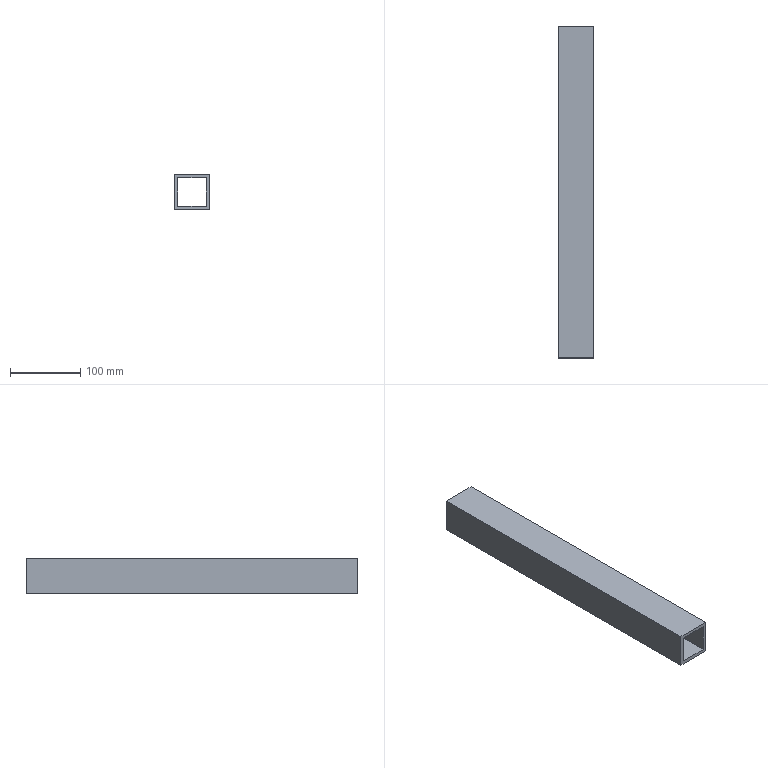Part | NX | features solid 2 | 1 solid | 10 faces | box 50 x 473 x 50 mm | volume 425700 mm3 | plane 10
STEP:
#1=CARTESIAN_POINT('',(1105.,523.,-520.));
#2=VERTEX_POINT('',#1);
#3=CARTESIAN_POINT('',(1105.,523.,-560.));
#4=VERTEX_POINT('',#3);
#5=CARTESIAN_POINT('',(1105.,523.,-520.));
#6=DIRECTION('',(0.,0.,-1.));
#7=VECTOR('',#6,1000.);
#8=LINE('',#5,#7);
#9=EDGE_CURVE('',#2,#4,#8,.T.);
#10=ORIENTED_EDGE('',*,*,#9,.F.);
#11=CARTESIAN_POINT('',(1065.,523.,-520.));
#12=VERTEX_POINT('',#11);
#13=CARTESIAN_POINT('',(1065.,523.,-520.));
#14=DIRECTION('',(1.,0.,0.));
#15=VECTOR('',#14,1000.);
#16=LINE('',#13,#15);
#17=EDGE_CURVE('',#12,#2,#16,.T.);
#18=ORIENTED_EDGE('',*,*,#17,.F.);
#19=CARTESIAN_POINT('',(1065.,523.,-560.));
#20=VERTEX_POINT('',#19);
#21=CARTESIAN_POINT('',(1065.,523.,-560.));
#22=DIRECTION('',(0.,0.,1.));
#23=VECTOR('',#22,1000.);
#24=LINE('',#21,#23);
#25=EDGE_CURVE('',#20,#12,#24,.T.);
#26=ORIENTED_EDGE('',*,*,#25,.F.);
#27=CARTESIAN_POINT('',(1105.,523.,-560.));
#28=DIRECTION('',(-1.,0.,0.));
#29=VECTOR('',#28,1000.);
#30=LINE('',#27,#29);
#31=EDGE_CURVE('',#4,#20,#30,.T.);
#32=ORIENTED_EDGE('',*,*,#31,.F.);
#33=EDGE_LOOP('',(#10,#18,#26,#32));
#34=FACE_BOUND('',#33,.T.);
#35=CARTESIAN_POINT('',(1110.,523.,-565.));
#36=VERTEX_POINT('',#35);
#37=CARTESIAN_POINT('',(1110.,523.,-515.));
#38=VERTEX_POINT('',#37);
#39=CARTESIAN_POINT('',(1110.,523.,-565.));
#40=DIRECTION('',(0.,0.,1.));
#41=VECTOR('',#40,1000.);
#42=LINE('',#39,#41);
#43=EDGE_CURVE('',#36,#38,#42,.T.);
#44=ORIENTED_EDGE('',*,*,#43,.F.);
#45=CARTESIAN_POINT('',(1060.,523.,-565.));
#46=VERTEX_POINT('',#45);
#47=CARTESIAN_POINT('',(1060.,523.,-565.));
#48=DIRECTION('',(1.,0.,0.));
#49=VECTOR('',#48,1000.);
#50=LINE('',#47,#49);
#51=EDGE_CURVE('',#46,#36,#50,.T.);
#52=ORIENTED_EDGE('',*,*,#51,.F.);
#53=CARTESIAN_POINT('',(1060.,523.,-515.));
#54=VERTEX_POINT('',#53);
#55=CARTESIAN_POINT('',(1060.,523.,-515.));
#56=DIRECTION('',(0.,0.,-1.));
#57=VECTOR('',#56,1000.);
#58=LINE('',#55,#57);
#59=EDGE_CURVE('',#54,#46,#58,.T.);
#60=ORIENTED_EDGE('',*,*,#59,.F.);
#61=CARTESIAN_POINT('',(1110.,523.,-515.));
#62=DIRECTION('',(-1.,0.,0.));
#63=VECTOR('',#62,1000.);
#64=LINE('',#61,#63);
#65=EDGE_CURVE('',#38,#54,#64,.T.);
#66=ORIENTED_EDGE('',*,*,#65,.F.);
#67=EDGE_LOOP('',(#44,#52,#60,#66));
#68=FACE_BOUND('',#67,.T.);
#69=CARTESIAN_POINT('',(1112.326,523.,-534.602));
#70=DIRECTION('',(0.,-1.,0.));
#71=DIRECTION('',(-1.,0.,0.));
#72=AXIS2_PLACEMENT_3D('',#69,#70,#71);
#73=PLANE('',#72);
#74=ADVANCED_FACE('',(#34,#68),#73,.F.);
#75=CARTESIAN_POINT('',(1105.,50.,-520.));
#76=VERTEX_POINT('',#75);
#77=CARTESIAN_POINT('',(1105.,50.,-560.));
#78=VERTEX_POINT('',#77);
#79=CARTESIAN_POINT('',(1105.,50.,-520.));
#80=DIRECTION('',(0.,0.,-1.));
#81=VECTOR('',#80,1000.);
#82=LINE('',#79,#81);
#83=EDGE_CURVE('',#76,#78,#82,.T.);
#84=ORIENTED_EDGE('',*,*,#83,.T.);
#85=CARTESIAN_POINT('',(1065.,50.,-560.));
#86=VERTEX_POINT('',#85);
#87=CARTESIAN_POINT('',(1105.,50.,-560.));
#88=DIRECTION('',(-1.,0.,0.));
#89=VECTOR('',#88,1000.);
#90=LINE('',#87,#89);
#91=EDGE_CURVE('',#78,#86,#90,.T.);
#92=ORIENTED_EDGE('',*,*,#91,.T.);
#93=CARTESIAN_POINT('',(1065.,50.,-520.));
#94=VERTEX_POINT('',#93);
#95=CARTESIAN_POINT('',(1065.,50.,-560.));
#96=DIRECTION('',(0.,0.,1.));
#97=VECTOR('',#96,1000.);
#98=LINE('',#95,#97);
#99=EDGE_CURVE('',#86,#94,#98,.T.);
#100=ORIENTED_EDGE('',*,*,#99,.T.);
#101=CARTESIAN_POINT('',(1065.,50.,-520.));
#102=DIRECTION('',(1.,0.,0.));
#103=VECTOR('',#102,1000.);
#104=LINE('',#101,#103);
#105=EDGE_CURVE('',#94,#76,#104,.T.);
#106=ORIENTED_EDGE('',*,*,#105,.T.);
#107=EDGE_LOOP('',(#84,#92,#100,#106));
#108=FACE_BOUND('',#107,.T.);
#109=CARTESIAN_POINT('',(1110.,50.,-565.));
#110=VERTEX_POINT('',#109);
#111=CARTESIAN_POINT('',(1110.,50.,-515.));
#112=VERTEX_POINT('',#111);
#113=CARTESIAN_POINT('',(1110.,50.,-565.));
#114=DIRECTION('',(0.,0.,1.));
#115=VECTOR('',#114,1000.);
#116=LINE('',#113,#115);
#117=EDGE_CURVE('',#110,#112,#116,.T.);
#118=ORIENTED_EDGE('',*,*,#117,.T.);
#119=CARTESIAN_POINT('',(1060.,50.,-515.));
#120=VERTEX_POINT('',#119);
#121=CARTESIAN_POINT('',(1110.,50.,-515.));
#122=DIRECTION('',(-1.,0.,0.));
#123=VECTOR('',#122,1000.);
#124=LINE('',#121,#123);
#125=EDGE_CURVE('',#112,#120,#124,.T.);
#126=ORIENTED_EDGE('',*,*,#125,.T.);
#127=CARTESIAN_POINT('',(1060.,50.,-565.));
#128=VERTEX_POINT('',#127);
#129=CARTESIAN_POINT('',(1060.,50.,-515.));
#130=DIRECTION('',(0.,0.,-1.));
#131=VECTOR('',#130,1000.);
#132=LINE('',#129,#131);
#133=EDGE_CURVE('',#120,#128,#132,.T.);
#134=ORIENTED_EDGE('',*,*,#133,.T.);
#135=CARTESIAN_POINT('',(1060.,50.,-565.));
#136=DIRECTION('',(1.,0.,0.));
#137=VECTOR('',#136,1000.);
#138=LINE('',#135,#137);
#139=EDGE_CURVE('',#128,#110,#138,.T.);
#140=ORIENTED_EDGE('',*,*,#139,.T.);
#141=EDGE_LOOP('',(#118,#126,#134,#140));
#142=FACE_BOUND('',#141,.T.);
#143=CARTESIAN_POINT('',(1112.326,50.,-534.602));
#144=DIRECTION('',(0.,-1.,0.));
#145=DIRECTION('',(-1.,0.,0.));
#146=AXIS2_PLACEMENT_3D('',#143,#144,#145);
#147=PLANE('',#146);
#148=ADVANCED_FACE('',(#108,#142),#147,.T.);
#149=ORIENTED_EDGE('',*,*,#17,.T.);
#150=CARTESIAN_POINT('',(1105.,45.,-520.));
#151=DIRECTION('',(0.,1.,0.));
#152=VECTOR('',#151,1000.);
#153=LINE('',#150,#152);
#154=EDGE_CURVE('',#76,#2,#153,.T.);
#155=ORIENTED_EDGE('',*,*,#154,.F.);
#156=ORIENTED_EDGE('',*,*,#105,.F.);
#157=CARTESIAN_POINT('',(1065.,45.,-520.));
#158=DIRECTION('',(0.,1.,0.));
#159=VECTOR('',#158,1000.);
#160=LINE('',#157,#159);
#161=EDGE_CURVE('',#94,#12,#160,.T.);
#162=ORIENTED_EDGE('',*,*,#161,.T.);
#163=EDGE_LOOP('',(#149,#155,#156,#162));
#164=FACE_BOUND('',#163,.T.);
#165=CARTESIAN_POINT('',(1065.,45.,-520.));
#166=DIRECTION('',(0.,0.,1.));
#167=DIRECTION('',(0.,-1.,0.));
#168=AXIS2_PLACEMENT_3D('',#165,#166,#167);
#169=PLANE('',#168);
#170=ADVANCED_FACE('',(#164),#169,.F.);
#171=ORIENTED_EDGE('',*,*,#51,.T.);
#172=CARTESIAN_POINT('',(1110.,45.,-565.));
#173=DIRECTION('',(0.,1.,0.));
#174=VECTOR('',#173,1000.);
#175=LINE('',#172,#174);
#176=EDGE_CURVE('',#110,#36,#175,.T.);
#177=ORIENTED_EDGE('',*,*,#176,.F.);
#178=ORIENTED_EDGE('',*,*,#139,.F.);
#179=CARTESIAN_POINT('',(1060.,45.,-565.));
#180=DIRECTION('',(0.,1.,0.));
#181=VECTOR('',#180,1000.);
#182=LINE('',#179,#181);
#183=EDGE_CURVE('',#128,#46,#182,.T.);
#184=ORIENTED_EDGE('',*,*,#183,.T.);
#185=EDGE_LOOP('',(#171,#177,#178,#184));
#186=FACE_BOUND('',#185,.T.);
#187=CARTESIAN_POINT('',(1060.,45.,-565.));
#188=DIRECTION('',(0.,0.,1.));
#189=DIRECTION('',(0.,-1.,0.));
#190=AXIS2_PLACEMENT_3D('',#187,#188,#189);
#191=PLANE('',#190);
#192=ADVANCED_FACE('',(#186),#191,.F.);
#193=ORIENTED_EDGE('',*,*,#59,.T.);
#194=ORIENTED_EDGE('',*,*,#183,.F.);
#195=ORIENTED_EDGE('',*,*,#133,.F.);
#196=CARTESIAN_POINT('',(1060.,45.,-515.));
#197=DIRECTION('',(0.,1.,0.));
#198=VECTOR('',#197,1000.);
#199=LINE('',#196,#198);
#200=EDGE_CURVE('',#120,#54,#199,.T.);
#201=ORIENTED_EDGE('',*,*,#200,.T.);
#202=EDGE_LOOP('',(#193,#194,#195,#201));
#203=FACE_BOUND('',#202,.T.);
#204=CARTESIAN_POINT('',(1060.,45.,-515.));
#205=DIRECTION('',(1.,0.,0.));
#206=DIRECTION('',(0.,-1.,0.));
#207=AXIS2_PLACEMENT_3D('',#204,#205,#206);
#208=PLANE('',#207);
#209=ADVANCED_FACE('',(#203),#208,.F.);
#210=ORIENTED_EDGE('',*,*,#65,.T.);
#211=ORIENTED_EDGE('',*,*,#200,.F.);
#212=ORIENTED_EDGE('',*,*,#125,.F.);
#213=CARTESIAN_POINT('',(1110.,45.,-515.));
#214=DIRECTION('',(0.,1.,0.));
#215=VECTOR('',#214,1000.);
#216=LINE('',#213,#215);
#217=EDGE_CURVE('',#112,#38,#216,.T.);
#218=ORIENTED_EDGE('',*,*,#217,.T.);
#219=EDGE_LOOP('',(#210,#211,#212,#218));
#220=FACE_BOUND('',#219,.T.);
#221=CARTESIAN_POINT('',(1110.,45.,-515.));
#222=DIRECTION('',(0.,0.,-1.));
#223=DIRECTION('',(-1.,0.,0.));
#224=AXIS2_PLACEMENT_3D('',#221,#222,#223);
#225=PLANE('',#224);
#226=ADVANCED_FACE('',(#220),#225,.F.);
#227=ORIENTED_EDGE('',*,*,#43,.T.);
#228=ORIENTED_EDGE('',*,*,#217,.F.);
#229=ORIENTED_EDGE('',*,*,#117,.F.);
#230=ORIENTED_EDGE('',*,*,#176,.T.);
#231=EDGE_LOOP('',(#227,#228,#229,#230));
#232=FACE_BOUND('',#231,.T.);
#233=CARTESIAN_POINT('',(1110.,45.,-565.));
#234=DIRECTION('',(-1.,0.,0.));
#235=DIRECTION('',(0.,0.,1.));
#236=AXIS2_PLACEMENT_3D('',#233,#234,#235);
#237=PLANE('',#236);
#238=ADVANCED_FACE('',(#232),#237,.F.);
#239=ORIENTED_EDGE('',*,*,#25,.T.);
#240=ORIENTED_EDGE('',*,*,#161,.F.);
#241=ORIENTED_EDGE('',*,*,#99,.F.);
#242=CARTESIAN_POINT('',(1065.,45.,-560.));
#243=DIRECTION('',(0.,1.,0.));
#244=VECTOR('',#243,1000.);
#245=LINE('',#242,#244);
#246=EDGE_CURVE('',#86,#20,#245,.T.);
#247=ORIENTED_EDGE('',*,*,#246,.T.);
#248=EDGE_LOOP('',(#239,#240,#241,#247));
#249=FACE_BOUND('',#248,.T.);
#250=CARTESIAN_POINT('',(1065.,45.,-560.));
#251=DIRECTION('',(-1.,0.,0.));
#252=DIRECTION('',(0.,0.,1.));
#253=AXIS2_PLACEMENT_3D('',#250,#251,#252);
#254=PLANE('',#253);
#255=ADVANCED_FACE('',(#249),#254,.F.);
#256=ORIENTED_EDGE('',*,*,#31,.T.);
#257=ORIENTED_EDGE('',*,*,#246,.F.);
#258=ORIENTED_EDGE('',*,*,#91,.F.);
#259=CARTESIAN_POINT('',(1105.,45.,-560.));
#260=DIRECTION('',(0.,1.,0.));
#261=VECTOR('',#260,1000.);
#262=LINE('',#259,#261);
#263=EDGE_CURVE('',#78,#4,#262,.T.);
#264=ORIENTED_EDGE('',*,*,#263,.T.);
#265=EDGE_LOOP('',(#256,#257,#258,#264));
#266=FACE_BOUND('',#265,.T.);
#267=CARTESIAN_POINT('',(1105.,45.,-560.));
#268=DIRECTION('',(0.,0.,-1.));
#269=DIRECTION('',(-1.,0.,0.));
#270=AXIS2_PLACEMENT_3D('',#267,#268,#269);
#271=PLANE('',#270);
#272=ADVANCED_FACE('',(#266),#271,.F.);
#273=ORIENTED_EDGE('',*,*,#9,.T.);
#274=ORIENTED_EDGE('',*,*,#263,.F.);
#275=ORIENTED_EDGE('',*,*,#83,.F.);
#276=ORIENTED_EDGE('',*,*,#154,.T.);
#277=EDGE_LOOP('',(#273,#274,#275,#276));
#278=FACE_BOUND('',#277,.T.);
#279=CARTESIAN_POINT('',(1105.,45.,-520.));
#280=DIRECTION('',(1.,0.,0.));
#281=DIRECTION('',(0.,-1.,0.));
#282=AXIS2_PLACEMENT_3D('',#279,#280,#281);
#283=PLANE('',#282);
#284=ADVANCED_FACE('',(#278),#283,.F.);
#285=CLOSED_SHELL('',(#74,#148,#170,#192,#209,#226,#238,#255,#272,#284));
#286=MANIFOLD_SOLID_BREP('',#285);
#287=(LENGTH_UNIT()NAMED_UNIT(*)SI_UNIT(.MILLI.,.METRE.));
#288=UNCERTAINTY_MEASURE_WITH_UNIT(LENGTH_MEASURE(0.00001),#287,'','');
#289=(NAMED_UNIT(*)PLANE_ANGLE_UNIT()SI_UNIT($,.RADIAN.));
#290=(NAMED_UNIT(*)SI_UNIT($,.STERADIAN.)SOLID_ANGLE_UNIT());
#291=(GEOMETRIC_REPRESENTATION_CONTEXT(3)GLOBAL_UNCERTAINTY_ASSIGNED_CONTEXT((#288))GLOBAL_UNIT_ASSIGNED_CONTEXT((#287,#289,#290))REPRESENTATION_CONTEXT('',''));
#292=ADVANCED_BREP_SHAPE_REPRESENTATION('',(#286),#291);